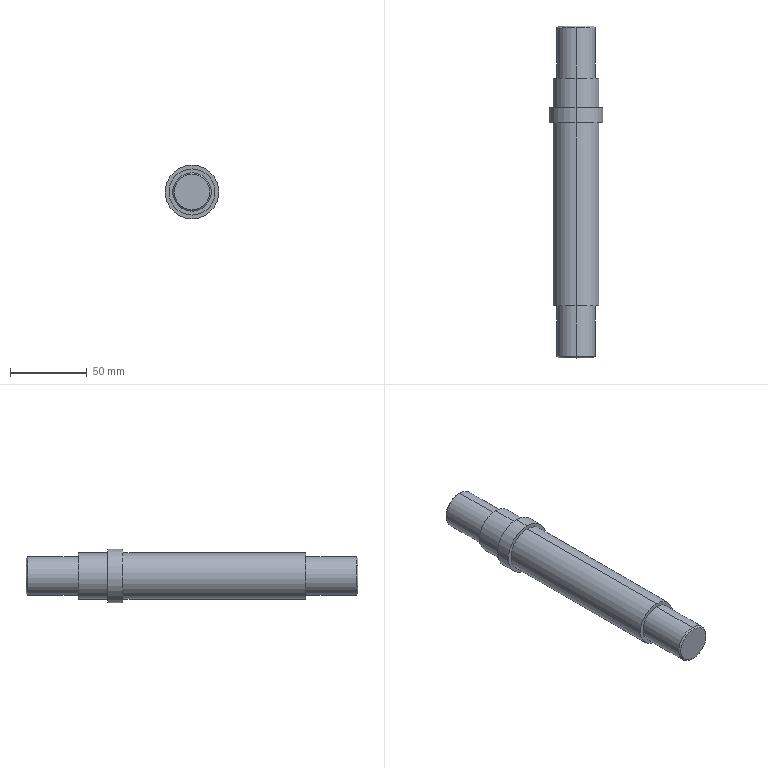Part | STEP file | 012-6-07-04 | 1 solid | 20 faces | box 35 x 216.4 x 35 mm | volume 140753 mm3 | cylinder 10 | plane 6 | cone 4 | commonest cylinder face diameters 25 x4 30 x4 35 x2
STEP:
#1=CARTESIAN_POINT('',(0.,0.,0.));
#2=DIRECTION('',(0.,0.,1.));
#3=DIRECTION('',(1.,0.,0.));
#4=AXIS2_PLACEMENT_3D('',#1,#2,#3);
#5=CARTESIAN_POINT('',(0.,216.4,11.5));
#6=VERTEX_POINT('',#5);
#7=CARTESIAN_POINT('',(0.,216.4,-11.5));
#8=VERTEX_POINT('',#7);
#9=CARTESIAN_POINT('',(0.,216.4,0.));
#10=DIRECTION('',(0.,1.,0.));
#11=DIRECTION('',(0.,0.,1.));
#12=AXIS2_PLACEMENT_3D('',#9,#10,#11);
#13=CIRCLE('',#12,11.5);
#14=CARTESIAN_POINT('',(0.,215.4,0.));
#15=DIRECTION('',(0.,-1.,0.));
#16=DIRECTION('',(0.,0.,-1.));
#17=AXIS2_PLACEMENT_3D('',#14,#15,#16);
#18=CONICAL_SURFACE('',#17,12.5,0.7854);
#19=CARTESIAN_POINT('',(3.142,-1.));
#20=DIRECTION('',(-1.,0.));
#21=VECTOR('',#20,1.);
#22=LINE('',#19,#21);
#23=(GEOMETRIC_REPRESENTATION_CONTEXT(2)PARAMETRIC_REPRESENTATION_CONTEXT()REPRESENTATION_CONTEXT('',''));
#24=DEFINITIONAL_REPRESENTATION('',(#22),#23);
#25=PCURVE('',#18,#24);
#26=CARTESIAN_POINT('',(12.5,216.4,0.));
#27=DIRECTION('',(0.,1.,0.));
#28=DIRECTION('',(0.,0.,1.));
#29=AXIS2_PLACEMENT_3D('',#26,#27,#28);
#30=PLANE('',#29);
#31=CARTESIAN_POINT('',(0.,-12.5));
#32=DIRECTION('',(1.,0.));
#33=AXIS2_PLACEMENT_2D('',#31,#32);
#34=CIRCLE('',#33,11.5);
#35=(GEOMETRIC_REPRESENTATION_CONTEXT(2)PARAMETRIC_REPRESENTATION_CONTEXT()REPRESENTATION_CONTEXT('',''));
#36=DEFINITIONAL_REPRESENTATION('',(#34),#35);
#37=PCURVE('',#30,#36);
#38=SURFACE_CURVE('',#13,(#25,#37),.PCURVE_S1.);
#39=EDGE_CURVE('',#6,#8,#38,.T.);
#40=ORIENTED_EDGE('',*,*,#39,.F.);
#41=CARTESIAN_POINT('',(0.,215.4,12.5));
#42=VERTEX_POINT('',#41);
#43=CARTESIAN_POINT('',(0.,215.4,12.5));
#44=DIRECTION('',(0.,-0.7071,0.7071));
#45=VECTOR('',#44,1.);
#46=LINE('',#43,#45);
#47=CARTESIAN_POINT('',(3.142,0.));
#48=DIRECTION('',(0.,1.));
#49=VECTOR('',#48,1.);
#50=LINE('',#47,#49);
#51=(GEOMETRIC_REPRESENTATION_CONTEXT(2)PARAMETRIC_REPRESENTATION_CONTEXT()REPRESENTATION_CONTEXT('',''));
#52=DEFINITIONAL_REPRESENTATION('',(#50),#51);
#53=PCURVE('',#18,#52);
#54=CARTESIAN_POINT('',(0.,215.4,0.));
#55=DIRECTION('',(0.,-1.,0.));
#56=DIRECTION('',(0.,0.,-1.));
#57=AXIS2_PLACEMENT_3D('',#54,#55,#56);
#58=CONICAL_SURFACE('',#57,12.5,0.7854);
#59=CARTESIAN_POINT('',(3.142,0.));
#60=DIRECTION('',(0.,1.));
#61=VECTOR('',#60,1.);
#62=LINE('',#59,#61);
#63=(GEOMETRIC_REPRESENTATION_CONTEXT(2)PARAMETRIC_REPRESENTATION_CONTEXT()REPRESENTATION_CONTEXT('',''));
#64=DEFINITIONAL_REPRESENTATION('',(#62),#63);
#65=PCURVE('',#58,#64);
#66=SURFACE_CURVE('',#46,(#53,#65),.PCURVE_S1.);
#67=EDGE_CURVE('',#6,#42,#66,.T.);
#68=ORIENTED_EDGE('',*,*,#67,.T.);
#69=CARTESIAN_POINT('',(0.,215.4,-12.5));
#70=VERTEX_POINT('',#69);
#71=CARTESIAN_POINT('',(0.,215.4,0.));
#72=DIRECTION('',(0.,-1.,0.));
#73=DIRECTION('',(0.,0.,1.));
#74=AXIS2_PLACEMENT_3D('',#71,#72,#73);
#75=CIRCLE('',#74,12.5);
#76=CARTESIAN_POINT('',(-3.142,0.));
#77=DIRECTION('',(1.,0.));
#78=VECTOR('',#77,1.);
#79=LINE('',#76,#78);
#80=(GEOMETRIC_REPRESENTATION_CONTEXT(2)PARAMETRIC_REPRESENTATION_CONTEXT()REPRESENTATION_CONTEXT('',''));
#81=DEFINITIONAL_REPRESENTATION('',(#79),#80);
#82=PCURVE('',#18,#81);
#83=CARTESIAN_POINT('',(0.,0.,0.));
#84=DIRECTION('',(0.,-1.,0.));
#85=DIRECTION('',(0.,0.,-1.));
#86=AXIS2_PLACEMENT_3D('',#83,#84,#85);
#87=CYLINDRICAL_SURFACE('',#86,12.5);
#88=CARTESIAN_POINT('',(-3.142,-215.4));
#89=DIRECTION('',(1.,0.));
#90=VECTOR('',#89,1.);
#91=LINE('',#88,#90);
#92=(GEOMETRIC_REPRESENTATION_CONTEXT(2)PARAMETRIC_REPRESENTATION_CONTEXT()REPRESENTATION_CONTEXT('',''));
#93=DEFINITIONAL_REPRESENTATION('',(#91),#92);
#94=PCURVE('',#87,#93);
#95=SURFACE_CURVE('',#75,(#82,#94),.PCURVE_S1.);
#96=EDGE_CURVE('',#70,#42,#95,.T.);
#97=ORIENTED_EDGE('',*,*,#96,.F.);
#98=CARTESIAN_POINT('',(0.,215.4,-12.5));
#99=DIRECTION('',(0.,-0.7071,-0.7071));
#100=VECTOR('',#99,1.);
#101=LINE('',#98,#100);
#102=CARTESIAN_POINT('',(0.,0.));
#103=DIRECTION('',(0.,1.));
#104=VECTOR('',#103,1.);
#105=LINE('',#102,#104);
#106=(GEOMETRIC_REPRESENTATION_CONTEXT(2)PARAMETRIC_REPRESENTATION_CONTEXT()REPRESENTATION_CONTEXT('',''));
#107=DEFINITIONAL_REPRESENTATION('',(#105),#106);
#108=PCURVE('',#18,#107);
#109=CARTESIAN_POINT('',(6.283,0.));
#110=DIRECTION('',(0.,1.));
#111=VECTOR('',#110,1.);
#112=LINE('',#109,#111);
#113=(GEOMETRIC_REPRESENTATION_CONTEXT(2)PARAMETRIC_REPRESENTATION_CONTEXT()REPRESENTATION_CONTEXT('',''));
#114=DEFINITIONAL_REPRESENTATION('',(#112),#113);
#115=PCURVE('',#58,#114);
#116=SURFACE_CURVE('',#101,(#108,#115),.PCURVE_S1.);
#117=EDGE_CURVE('',#8,#70,#116,.T.);
#118=ORIENTED_EDGE('',*,*,#117,.F.);
#119=EDGE_LOOP('',(#40,#68,#97,#118));
#120=FACE_BOUND('',#119,.T.);
#121=ADVANCED_FACE('',(#120),#18,.T.);
#122=CARTESIAN_POINT('',(0.,0.,-11.5));
#123=VERTEX_POINT('',#122);
#124=CARTESIAN_POINT('',(0.,0.,11.5));
#125=VERTEX_POINT('',#124);
#126=CARTESIAN_POINT('',(0.,0.,0.));
#127=DIRECTION('',(0.,-1.,0.));
#128=DIRECTION('',(0.,0.,-1.));
#129=AXIS2_PLACEMENT_3D('',#126,#127,#128);
#130=CIRCLE('',#129,11.5);
#131=CARTESIAN_POINT('',(0.,0.,0.));
#132=DIRECTION('',(0.,1.,0.));
#133=DIRECTION('',(0.,0.,1.));
#134=AXIS2_PLACEMENT_3D('',#131,#132,#133);
#135=CONICAL_SURFACE('',#134,11.5,0.7854);
#136=CARTESIAN_POINT('',(3.142,0.));
#137=DIRECTION('',(-1.,0.));
#138=VECTOR('',#137,1.);
#139=LINE('',#136,#138);
#140=(GEOMETRIC_REPRESENTATION_CONTEXT(2)PARAMETRIC_REPRESENTATION_CONTEXT()REPRESENTATION_CONTEXT('',''));
#141=DEFINITIONAL_REPRESENTATION('',(#139),#140);
#142=PCURVE('',#135,#141);
#143=CARTESIAN_POINT('',(0.,0.,0.));
#144=DIRECTION('',(0.,-1.,0.));
#145=DIRECTION('',(0.,0.,-1.));
#146=AXIS2_PLACEMENT_3D('',#143,#144,#145);
#147=PLANE('',#146);
#148=CARTESIAN_POINT('',(0.,0.));
#149=DIRECTION('',(1.,0.));
#150=AXIS2_PLACEMENT_2D('',#148,#149);
#151=CIRCLE('',#150,11.5);
#152=(GEOMETRIC_REPRESENTATION_CONTEXT(2)PARAMETRIC_REPRESENTATION_CONTEXT()REPRESENTATION_CONTEXT('',''));
#153=DEFINITIONAL_REPRESENTATION('',(#151),#152);
#154=PCURVE('',#147,#153);
#155=SURFACE_CURVE('',#130,(#142,#154),.PCURVE_S1.);
#156=EDGE_CURVE('',#123,#125,#155,.T.);
#157=ORIENTED_EDGE('',*,*,#156,.F.);
#158=CARTESIAN_POINT('',(0.,1.,-12.5));
#159=VERTEX_POINT('',#158);
#160=CARTESIAN_POINT('',(0.,0.,-11.5));
#161=DIRECTION('',(0.,0.7071,-0.7071));
#162=VECTOR('',#161,1.);
#163=LINE('',#160,#162);
#164=CARTESIAN_POINT('',(3.142,0.));
#165=DIRECTION('',(0.,1.));
#166=VECTOR('',#165,1.);
#167=LINE('',#164,#166);
#168=(GEOMETRIC_REPRESENTATION_CONTEXT(2)PARAMETRIC_REPRESENTATION_CONTEXT()REPRESENTATION_CONTEXT('',''));
#169=DEFINITIONAL_REPRESENTATION('',(#167),#168);
#170=PCURVE('',#135,#169);
#171=CARTESIAN_POINT('',(0.,0.,0.));
#172=DIRECTION('',(0.,1.,0.));
#173=DIRECTION('',(0.,0.,1.));
#174=AXIS2_PLACEMENT_3D('',#171,#172,#173);
#175=CONICAL_SURFACE('',#174,11.5,0.7854);
#176=CARTESIAN_POINT('',(3.142,0.));
#177=DIRECTION('',(0.,1.));
#178=VECTOR('',#177,1.);
#179=LINE('',#176,#178);
#180=(GEOMETRIC_REPRESENTATION_CONTEXT(2)PARAMETRIC_REPRESENTATION_CONTEXT()REPRESENTATION_CONTEXT('',''));
#181=DEFINITIONAL_REPRESENTATION('',(#179),#180);
#182=PCURVE('',#175,#181);
#183=SURFACE_CURVE('',#163,(#170,#182),.PCURVE_S1.);
#184=EDGE_CURVE('',#123,#159,#183,.T.);
#185=ORIENTED_EDGE('',*,*,#184,.T.);
#186=CARTESIAN_POINT('',(0.,1.,12.5));
#187=VERTEX_POINT('',#186);
#188=CARTESIAN_POINT('',(0.,1.,0.));
#189=DIRECTION('',(0.,1.,0.));
#190=DIRECTION('',(0.,0.,-1.));
#191=AXIS2_PLACEMENT_3D('',#188,#189,#190);
#192=CIRCLE('',#191,12.5);
#193=CARTESIAN_POINT('',(-3.142,1.));
#194=DIRECTION('',(1.,0.));
#195=VECTOR('',#194,1.);
#196=LINE('',#193,#195);
#197=(GEOMETRIC_REPRESENTATION_CONTEXT(2)PARAMETRIC_REPRESENTATION_CONTEXT()REPRESENTATION_CONTEXT('',''));
#198=DEFINITIONAL_REPRESENTATION('',(#196),#197);
#199=PCURVE('',#135,#198);
#200=CARTESIAN_POINT('',(0.,0.,0.));
#201=DIRECTION('',(0.,-1.,0.));
#202=DIRECTION('',(0.,0.,-1.));
#203=AXIS2_PLACEMENT_3D('',#200,#201,#202);
#204=CYLINDRICAL_SURFACE('',#203,12.5);
#205=CARTESIAN_POINT('',(6.283,-1.));
#206=DIRECTION('',(-1.,0.));
#207=VECTOR('',#206,1.);
#208=LINE('',#205,#207);
#209=(GEOMETRIC_REPRESENTATION_CONTEXT(2)PARAMETRIC_REPRESENTATION_CONTEXT()REPRESENTATION_CONTEXT('',''));
#210=DEFINITIONAL_REPRESENTATION('',(#208),#209);
#211=PCURVE('',#204,#210);
#212=SURFACE_CURVE('',#192,(#199,#211),.PCURVE_S1.);
#213=EDGE_CURVE('',#187,#159,#212,.T.);
#214=ORIENTED_EDGE('',*,*,#213,.F.);
#215=CARTESIAN_POINT('',(0.,0.,11.5));
#216=DIRECTION('',(0.,0.7071,0.7071));
#217=VECTOR('',#216,1.);
#218=LINE('',#215,#217);
#219=CARTESIAN_POINT('',(0.,0.));
#220=DIRECTION('',(0.,1.));
#221=VECTOR('',#220,1.);
#222=LINE('',#219,#221);
#223=(GEOMETRIC_REPRESENTATION_CONTEXT(2)PARAMETRIC_REPRESENTATION_CONTEXT()REPRESENTATION_CONTEXT('',''));
#224=DEFINITIONAL_REPRESENTATION('',(#222),#223);
#225=PCURVE('',#135,#224);
#226=CARTESIAN_POINT('',(6.283,0.));
#227=DIRECTION('',(0.,1.));
#228=VECTOR('',#227,1.);
#229=LINE('',#226,#228);
#230=(GEOMETRIC_REPRESENTATION_CONTEXT(2)PARAMETRIC_REPRESENTATION_CONTEXT()REPRESENTATION_CONTEXT('',''));
#231=DEFINITIONAL_REPRESENTATION('',(#229),#230);
#232=PCURVE('',#175,#231);
#233=SURFACE_CURVE('',#218,(#225,#232),.PCURVE_S1.);
#234=EDGE_CURVE('',#125,#187,#233,.T.);
#235=ORIENTED_EDGE('',*,*,#234,.F.);
#236=EDGE_LOOP('',(#157,#185,#214,#235));
#237=FACE_BOUND('',#236,.T.);
#238=ADVANCED_FACE('',(#237),#135,.T.);
#239=ORIENTED_EDGE('',*,*,#96,.T.);
#240=CARTESIAN_POINT('',(0.,182.4,12.5));
#241=VERTEX_POINT('',#240);
#242=CARTESIAN_POINT('',(0.,0.,12.5));
#243=DIRECTION('',(0.,-1.,0.));
#244=VECTOR('',#243,1.);
#245=LINE('',#242,#244);
#246=CARTESIAN_POINT('',(3.142,0.));
#247=DIRECTION('',(0.,1.));
#248=VECTOR('',#247,1.);
#249=LINE('',#246,#248);
#250=(GEOMETRIC_REPRESENTATION_CONTEXT(2)PARAMETRIC_REPRESENTATION_CONTEXT()REPRESENTATION_CONTEXT('',''));
#251=DEFINITIONAL_REPRESENTATION('',(#249),#250);
#252=PCURVE('',#87,#251);
#253=CARTESIAN_POINT('',(0.,0.,0.));
#254=DIRECTION('',(0.,-1.,0.));
#255=DIRECTION('',(0.,0.,-1.));
#256=AXIS2_PLACEMENT_3D('',#253,#254,#255);
#257=CYLINDRICAL_SURFACE('',#256,12.5);
#258=CARTESIAN_POINT('',(3.142,0.));
#259=DIRECTION('',(0.,1.));
#260=VECTOR('',#259,1.);
#261=LINE('',#258,#260);
#262=(GEOMETRIC_REPRESENTATION_CONTEXT(2)PARAMETRIC_REPRESENTATION_CONTEXT()REPRESENTATION_CONTEXT('',''));
#263=DEFINITIONAL_REPRESENTATION('',(#261),#262);
#264=PCURVE('',#257,#263);
#265=SURFACE_CURVE('',#245,(#252,#264),.PCURVE_S1.);
#266=EDGE_CURVE('',#42,#241,#265,.T.);
#267=ORIENTED_EDGE('',*,*,#266,.T.);
#268=CARTESIAN_POINT('',(0.,182.4,-12.5));
#269=VERTEX_POINT('',#268);
#270=CARTESIAN_POINT('',(0.,182.4,0.));
#271=DIRECTION('',(0.,-1.,0.));
#272=DIRECTION('',(0.,0.,-1.));
#273=AXIS2_PLACEMENT_3D('',#270,#271,#272);
#274=CIRCLE('',#273,12.5);
#275=CARTESIAN_POINT('',(0.,-182.4));
#276=DIRECTION('',(1.,0.));
#277=VECTOR('',#276,1.);
#278=LINE('',#275,#277);
#279=(GEOMETRIC_REPRESENTATION_CONTEXT(2)PARAMETRIC_REPRESENTATION_CONTEXT()REPRESENTATION_CONTEXT('',''));
#280=DEFINITIONAL_REPRESENTATION('',(#278),#279);
#281=PCURVE('',#87,#280);
#282=CARTESIAN_POINT('',(12.5,182.4,0.));
#283=DIRECTION('',(0.,1.,0.));
#284=DIRECTION('',(0.,0.,1.));
#285=AXIS2_PLACEMENT_3D('',#282,#283,#284);
#286=PLANE('',#285);
#287=CARTESIAN_POINT('',(-12.5,-12.5));
#288=CARTESIAN_POINT('',(-12.5,9.151));
#289=CARTESIAN_POINT('',(6.25,-1.675));
#290=CARTESIAN_POINT('',(25.,-12.5));
#291=CARTESIAN_POINT('',(6.25,-23.325));
#292=CARTESIAN_POINT('',(-12.5,-34.151));
#293=CARTESIAN_POINT('',(-12.5,-12.5));
#294=(BOUNDED_CURVE()B_SPLINE_CURVE(2,(#287,#288,#289,#290,#291,#292,#293),.UNSPECIFIED.,.T.,.F.)B_SPLINE_CURVE_WITH_KNOTS((1,2,2,2,2,1),(-2.094,0.,2.094,4.189,6.283,8.378),.UNSPECIFIED.)CURVE()GEOMETRIC_REPRESENTATION_ITEM()RATIONAL_B_SPLINE_CURVE((1.,0.5,1.,0.5,1.,0.5,1.))REPRESENTATION_ITEM(''));
#295=(GEOMETRIC_REPRESENTATION_CONTEXT(2)PARAMETRIC_REPRESENTATION_CONTEXT()REPRESENTATION_CONTEXT('',''));
#296=DEFINITIONAL_REPRESENTATION('',(#294),#295);
#297=PCURVE('',#286,#296);
#298=SURFACE_CURVE('',#274,(#281,#297),.PCURVE_S1.);
#299=EDGE_CURVE('',#269,#241,#298,.T.);
#300=ORIENTED_EDGE('',*,*,#299,.F.);
#301=CARTESIAN_POINT('',(0.,0.,-12.5));
#302=DIRECTION('',(0.,-1.,0.));
#303=VECTOR('',#302,1.);
#304=LINE('',#301,#303);
#305=CARTESIAN_POINT('',(0.,0.));
#306=DIRECTION('',(0.,1.));
#307=VECTOR('',#306,1.);
#308=LINE('',#305,#307);
#309=(GEOMETRIC_REPRESENTATION_CONTEXT(2)PARAMETRIC_REPRESENTATION_CONTEXT()REPRESENTATION_CONTEXT('',''));
#310=DEFINITIONAL_REPRESENTATION('',(#308),#309);
#311=PCURVE('',#87,#310);
#312=CARTESIAN_POINT('',(6.283,0.));
#313=DIRECTION('',(0.,1.));
#314=VECTOR('',#313,1.);
#315=LINE('',#312,#314);
#316=(GEOMETRIC_REPRESENTATION_CONTEXT(2)PARAMETRIC_REPRESENTATION_CONTEXT()REPRESENTATION_CONTEXT('',''));
#317=DEFINITIONAL_REPRESENTATION('',(#315),#316);
#318=PCURVE('',#257,#317);
#319=SURFACE_CURVE('',#304,(#311,#318),.PCURVE_S1.);
#320=EDGE_CURVE('',#70,#269,#319,.T.);
#321=ORIENTED_EDGE('',*,*,#320,.F.);
#322=EDGE_LOOP('',(#239,#267,#300,#321));
#323=FACE_BOUND('',#322,.T.);
#324=ADVANCED_FACE('',(#323),#87,.T.);
#325=CARTESIAN_POINT('',(0.,182.4,-15.));
#326=VERTEX_POINT('',#325);
#327=CARTESIAN_POINT('',(0.,182.4,15.));
#328=VERTEX_POINT('',#327);
#329=CARTESIAN_POINT('',(0.,182.4,0.));
#330=DIRECTION('',(0.,-1.,0.));
#331=DIRECTION('',(0.,0.,-1.));
#332=AXIS2_PLACEMENT_3D('',#329,#330,#331);
#333=CIRCLE('',#332,15.);
#334=CARTESIAN_POINT('',(0.,0.,0.));
#335=DIRECTION('',(0.,-1.,0.));
#336=DIRECTION('',(0.,0.,-1.));
#337=AXIS2_PLACEMENT_3D('',#334,#335,#336);
#338=CYLINDRICAL_SURFACE('',#337,15.);
#339=CARTESIAN_POINT('',(0.,-182.4));
#340=DIRECTION('',(1.,0.));
#341=VECTOR('',#340,1.);
#342=LINE('',#339,#341);
#343=(GEOMETRIC_REPRESENTATION_CONTEXT(2)PARAMETRIC_REPRESENTATION_CONTEXT()REPRESENTATION_CONTEXT('',''));
#344=DEFINITIONAL_REPRESENTATION('',(#342),#343);
#345=PCURVE('',#338,#344);
#346=CARTESIAN_POINT('',(-15.,-12.5));
#347=CARTESIAN_POINT('',(-15.,13.481));
#348=CARTESIAN_POINT('',(7.5,0.4904));
#349=CARTESIAN_POINT('',(30.,-12.5));
#350=CARTESIAN_POINT('',(7.5,-25.49));
#351=CARTESIAN_POINT('',(-15.,-38.481));
#352=CARTESIAN_POINT('',(-15.,-12.5));
#353=(BOUNDED_CURVE()B_SPLINE_CURVE(2,(#346,#347,#348,#349,#350,#351,#352),.UNSPECIFIED.,.T.,.F.)B_SPLINE_CURVE_WITH_KNOTS((1,2,2,2,2,1),(-2.094,0.,2.094,4.189,6.283,8.378),.UNSPECIFIED.)CURVE()GEOMETRIC_REPRESENTATION_ITEM()RATIONAL_B_SPLINE_CURVE((1.,0.5,1.,0.5,1.,0.5,1.))REPRESENTATION_ITEM(''));
#354=(GEOMETRIC_REPRESENTATION_CONTEXT(2)PARAMETRIC_REPRESENTATION_CONTEXT()REPRESENTATION_CONTEXT('',''));
#355=DEFINITIONAL_REPRESENTATION('',(#353),#354);
#356=PCURVE('',#286,#355);
#357=SURFACE_CURVE('',#333,(#345,#356),.PCURVE_S1.);
#358=EDGE_CURVE('',#326,#328,#357,.T.);
#359=ORIENTED_EDGE('',*,*,#358,.T.);
#360=CARTESIAN_POINT('',(0.,163.2,15.));
#361=VERTEX_POINT('',#360);
#362=CARTESIAN_POINT('',(0.,0.,15.));
#363=DIRECTION('',(0.,-1.,0.));
#364=VECTOR('',#363,1.);
#365=LINE('',#362,#364);
#366=CARTESIAN_POINT('',(3.142,0.));
#367=DIRECTION('',(0.,1.));
#368=VECTOR('',#367,1.);
#369=LINE('',#366,#368);
#370=(GEOMETRIC_REPRESENTATION_CONTEXT(2)PARAMETRIC_REPRESENTATION_CONTEXT()REPRESENTATION_CONTEXT('',''));
#371=DEFINITIONAL_REPRESENTATION('',(#369),#370);
#372=PCURVE('',#338,#371);
#373=CARTESIAN_POINT('',(0.,0.,0.));
#374=DIRECTION('',(0.,-1.,0.));
#375=DIRECTION('',(0.,0.,-1.));
#376=AXIS2_PLACEMENT_3D('',#373,#374,#375);
#377=CYLINDRICAL_SURFACE('',#376,15.);
#378=CARTESIAN_POINT('',(3.142,0.));
#379=DIRECTION('',(0.,1.));
#380=VECTOR('',#379,1.);
#381=LINE('',#378,#380);
#382=(GEOMETRIC_REPRESENTATION_CONTEXT(2)PARAMETRIC_REPRESENTATION_CONTEXT()REPRESENTATION_CONTEXT('',''));
#383=DEFINITIONAL_REPRESENTATION('',(#381),#382);
#384=PCURVE('',#377,#383);
#385=SURFACE_CURVE('',#365,(#372,#384),.PCURVE_S1.);
#386=EDGE_CURVE('',#328,#361,#385,.T.);
#387=ORIENTED_EDGE('',*,*,#386,.T.);
#388=CARTESIAN_POINT('',(0.,163.2,-15.));
#389=VERTEX_POINT('',#388);
#390=CARTESIAN_POINT('',(0.,163.2,0.));
#391=DIRECTION('',(0.,-1.,0.));
#392=DIRECTION('',(0.,0.,-1.));
#393=AXIS2_PLACEMENT_3D('',#390,#391,#392);
#394=CIRCLE('',#393,15.);
#395=CARTESIAN_POINT('',(0.,-163.2));
#396=DIRECTION('',(1.,0.));
#397=VECTOR('',#396,1.);
#398=LINE('',#395,#397);
#399=(GEOMETRIC_REPRESENTATION_CONTEXT(2)PARAMETRIC_REPRESENTATION_CONTEXT()REPRESENTATION_CONTEXT('',''));
#400=DEFINITIONAL_REPRESENTATION('',(#398),#399);
#401=PCURVE('',#338,#400);
#402=CARTESIAN_POINT('',(15.,163.2,0.));
#403=DIRECTION('',(0.,1.,0.));
#404=DIRECTION('',(0.,0.,1.));
#405=AXIS2_PLACEMENT_3D('',#402,#403,#404);
#406=PLANE('',#405);
#407=CARTESIAN_POINT('',(-15.,-15.));
#408=CARTESIAN_POINT('',(-15.,10.981));
#409=CARTESIAN_POINT('',(7.5,-2.01));
#410=CARTESIAN_POINT('',(30.,-15.));
#411=CARTESIAN_POINT('',(7.5,-27.99));
#412=CARTESIAN_POINT('',(-15.,-40.981));
#413=CARTESIAN_POINT('',(-15.,-15.));
#414=(BOUNDED_CURVE()B_SPLINE_CURVE(2,(#407,#408,#409,#410,#411,#412,#413),.UNSPECIFIED.,.T.,.F.)B_SPLINE_CURVE_WITH_KNOTS((1,2,2,2,2,1),(-2.094,0.,2.094,4.189,6.283,8.378),.UNSPECIFIED.)CURVE()GEOMETRIC_REPRESENTATION_ITEM()RATIONAL_B_SPLINE_CURVE((1.,0.5,1.,0.5,1.,0.5,1.))REPRESENTATION_ITEM(''));
#415=(GEOMETRIC_REPRESENTATION_CONTEXT(2)PARAMETRIC_REPRESENTATION_CONTEXT()REPRESENTATION_CONTEXT('',''));
#416=DEFINITIONAL_REPRESENTATION('',(#414),#415);
#417=PCURVE('',#406,#416);
#418=SURFACE_CURVE('',#394,(#401,#417),.PCURVE_S1.);
#419=EDGE_CURVE('',#389,#361,#418,.T.);
#420=ORIENTED_EDGE('',*,*,#419,.F.);
#421=CARTESIAN_POINT('',(0.,0.,-15.));
#422=DIRECTION('',(0.,-1.,0.));
#423=VECTOR('',#422,1.);
#424=LINE('',#421,#423);
#425=CARTESIAN_POINT('',(0.,0.));
#426=DIRECTION('',(0.,1.));
#427=VECTOR('',#426,1.);
#428=LINE('',#425,#427);
#429=(GEOMETRIC_REPRESENTATION_CONTEXT(2)PARAMETRIC_REPRESENTATION_CONTEXT()REPRESENTATION_CONTEXT('',''));
#430=DEFINITIONAL_REPRESENTATION('',(#428),#429);
#431=PCURVE('',#338,#430);
#432=CARTESIAN_POINT('',(6.283,0.));
#433=DIRECTION('',(0.,1.));
#434=VECTOR('',#433,1.);
#435=LINE('',#432,#434);
#436=(GEOMETRIC_REPRESENTATION_CONTEXT(2)PARAMETRIC_REPRESENTATION_CONTEXT()REPRESENTATION_CONTEXT('',''));
#437=DEFINITIONAL_REPRESENTATION('',(#435),#436);
#438=PCURVE('',#377,#437);
#439=SURFACE_CURVE('',#424,(#431,#438),.PCURVE_S1.);
#440=EDGE_CURVE('',#326,#389,#439,.T.);
#441=ORIENTED_EDGE('',*,*,#440,.F.);
#442=EDGE_LOOP('',(#359,#387,#420,#441));
#443=FACE_BOUND('',#442,.T.);
#444=ADVANCED_FACE('',(#443),#338,.T.);
#445=CARTESIAN_POINT('',(0.,163.2,-17.5));
#446=VERTEX_POINT('',#445);
#447=CARTESIAN_POINT('',(0.,163.2,17.5));
#448=VERTEX_POINT('',#447);
#449=CARTESIAN_POINT('',(0.,163.2,0.));
#450=DIRECTION('',(0.,-1.,0.));
#451=DIRECTION('',(0.,0.,-1.));
#452=AXIS2_PLACEMENT_3D('',#449,#450,#451);
#453=CIRCLE('',#452,17.5);
#454=CARTESIAN_POINT('',(0.,0.,0.));
#455=DIRECTION('',(0.,-1.,0.));
#456=DIRECTION('',(0.,0.,-1.));
#457=AXIS2_PLACEMENT_3D('',#454,#455,#456);
#458=CYLINDRICAL_SURFACE('',#457,17.5);
#459=CARTESIAN_POINT('',(0.,-163.2));
#460=DIRECTION('',(1.,0.));
#461=VECTOR('',#460,1.);
#462=LINE('',#459,#461);
#463=(GEOMETRIC_REPRESENTATION_CONTEXT(2)PARAMETRIC_REPRESENTATION_CONTEXT()REPRESENTATION_CONTEXT('',''));
#464=DEFINITIONAL_REPRESENTATION('',(#462),#463);
#465=PCURVE('',#458,#464);
#466=CARTESIAN_POINT('',(-17.5,-15.));
#467=CARTESIAN_POINT('',(-17.5,15.311));
#468=CARTESIAN_POINT('',(8.75,0.1554));
#469=CARTESIAN_POINT('',(35.,-15.));
#470=CARTESIAN_POINT('',(8.75,-30.155));
#471=CARTESIAN_POINT('',(-17.5,-45.311));
#472=CARTESIAN_POINT('',(-17.5,-15.));
#473=(BOUNDED_CURVE()B_SPLINE_CURVE(2,(#466,#467,#468,#469,#470,#471,#472),.UNSPECIFIED.,.T.,.F.)B_SPLINE_CURVE_WITH_KNOTS((1,2,2,2,2,1),(-2.094,0.,2.094,4.189,6.283,8.378),.UNSPECIFIED.)CURVE()GEOMETRIC_REPRESENTATION_ITEM()RATIONAL_B_SPLINE_CURVE((1.,0.5,1.,0.5,1.,0.5,1.))REPRESENTATION_ITEM(''));
#474=(GEOMETRIC_REPRESENTATION_CONTEXT(2)PARAMETRIC_REPRESENTATION_CONTEXT()REPRESENTATION_CONTEXT('',''));
#475=DEFINITIONAL_REPRESENTATION('',(#473),#474);
#476=PCURVE('',#406,#475);
#477=SURFACE_CURVE('',#453,(#465,#476),.PCURVE_S1.);
#478=EDGE_CURVE('',#446,#448,#477,.T.);
#479=ORIENTED_EDGE('',*,*,#478,.T.);
#480=CARTESIAN_POINT('',(0.,153.2,17.5));
#481=VERTEX_POINT('',#480);
#482=CARTESIAN_POINT('',(0.,0.,17.5));
#483=DIRECTION('',(0.,-1.,0.));
#484=VECTOR('',#483,1.);
#485=LINE('',#482,#484);
#486=CARTESIAN_POINT('',(3.142,0.));
#487=DIRECTION('',(0.,1.));
#488=VECTOR('',#487,1.);
#489=LINE('',#486,#488);
#490=(GEOMETRIC_REPRESENTATION_CONTEXT(2)PARAMETRIC_REPRESENTATION_CONTEXT()REPRESENTATION_CONTEXT('',''));
#491=DEFINITIONAL_REPRESENTATION('',(#489),#490);
#492=PCURVE('',#458,#491);
#493=CARTESIAN_POINT('',(0.,0.,0.));
#494=DIRECTION('',(0.,-1.,0.));
#495=DIRECTION('',(0.,0.,-1.));
#496=AXIS2_PLACEMENT_3D('',#493,#494,#495);
#497=CYLINDRICAL_SURFACE('',#496,17.5);
#498=CARTESIAN_POINT('',(3.142,0.));
#499=DIRECTION('',(0.,1.));
#500=VECTOR('',#499,1.);
#501=LINE('',#498,#500);
#502=(GEOMETRIC_REPRESENTATION_CONTEXT(2)PARAMETRIC_REPRESENTATION_CONTEXT()REPRESENTATION_CONTEXT('',''));
#503=DEFINITIONAL_REPRESENTATION('',(#501),#502);
#504=PCURVE('',#497,#503);
#505=SURFACE_CURVE('',#485,(#492,#504),.PCURVE_S1.);
#506=EDGE_CURVE('',#448,#481,#505,.T.);
#507=ORIENTED_EDGE('',*,*,#506,.T.);
#508=CARTESIAN_POINT('',(0.,153.2,-17.5));
#509=VERTEX_POINT('',#508);
#510=CARTESIAN_POINT('',(0.,153.2,0.));
#511=DIRECTION('',(0.,-1.,0.));
#512=DIRECTION('',(0.,0.,-1.));
#513=AXIS2_PLACEMENT_3D('',#510,#511,#512);
#514=CIRCLE('',#513,17.5);
#515=CARTESIAN_POINT('',(0.,-153.2));
#516=DIRECTION('',(1.,0.));
#517=VECTOR('',#516,1.);
#518=LINE('',#515,#517);
#519=(GEOMETRIC_REPRESENTATION_CONTEXT(2)PARAMETRIC_REPRESENTATION_CONTEXT()REPRESENTATION_CONTEXT('',''));
#520=DEFINITIONAL_REPRESENTATION('',(#518),#519);
#521=PCURVE('',#458,#520);
#522=CARTESIAN_POINT('',(15.,153.2,0.));
#523=DIRECTION('',(0.,-1.,0.));
#524=DIRECTION('',(0.,0.,-1.));
#525=AXIS2_PLACEMENT_3D('',#522,#523,#524);
#526=PLANE('',#525);
#527=CARTESIAN_POINT('',(0.,-15.));
#528=DIRECTION('',(1.,0.));
#529=AXIS2_PLACEMENT_2D('',#527,#528);
#530=CIRCLE('',#529,17.5);
#531=(GEOMETRIC_REPRESENTATION_CONTEXT(2)PARAMETRIC_REPRESENTATION_CONTEXT()REPRESENTATION_CONTEXT('',''));
#532=DEFINITIONAL_REPRESENTATION('',(#530),#531);
#533=PCURVE('',#526,#532);
#534=SURFACE_CURVE('',#514,(#521,#533),.PCURVE_S1.);
#535=EDGE_CURVE('',#509,#481,#534,.T.);
#536=ORIENTED_EDGE('',*,*,#535,.F.);
#537=CARTESIAN_POINT('',(0.,0.,-17.5));
#538=DIRECTION('',(0.,-1.,0.));
#539=VECTOR('',#538,1.);
#540=LINE('',#537,#539);
#541=CARTESIAN_POINT('',(0.,0.));
#542=DIRECTION('',(0.,1.));
#543=VECTOR('',#542,1.);
#544=LINE('',#541,#543);
#545=(GEOMETRIC_REPRESENTATION_CONTEXT(2)PARAMETRIC_REPRESENTATION_CONTEXT()REPRESENTATION_CONTEXT('',''));
#546=DEFINITIONAL_REPRESENTATION('',(#544),#545);
#547=PCURVE('',#458,#546);
#548=CARTESIAN_POINT('',(6.283,0.));
#549=DIRECTION('',(0.,1.));
#550=VECTOR('',#549,1.);
#551=LINE('',#548,#550);
#552=(GEOMETRIC_REPRESENTATION_CONTEXT(2)PARAMETRIC_REPRESENTATION_CONTEXT()REPRESENTATION_CONTEXT('',''));
#553=DEFINITIONAL_REPRESENTATION('',(#551),#552);
#554=PCURVE('',#497,#553);
#555=SURFACE_CURVE('',#540,(#547,#554),.PCURVE_S1.);
#556=EDGE_CURVE('',#446,#509,#555,.T.);
#557=ORIENTED_EDGE('',*,*,#556,.F.);
#558=EDGE_LOOP('',(#479,#507,#536,#557));
#559=FACE_BOUND('',#558,.T.);
#560=ADVANCED_FACE('',(#559),#458,.T.);
#561=CARTESIAN_POINT('',(0.,153.2,-15.));
#562=VERTEX_POINT('',#561);
#563=CARTESIAN_POINT('',(0.,153.2,15.));
#564=VERTEX_POINT('',#563);
#565=CARTESIAN_POINT('',(0.,153.2,0.));
#566=DIRECTION('',(0.,-1.,0.));
#567=DIRECTION('',(0.,0.,-1.));
#568=AXIS2_PLACEMENT_3D('',#565,#566,#567);
#569=CIRCLE('',#568,15.);
#570=CARTESIAN_POINT('',(0.,0.,0.));
#571=DIRECTION('',(0.,-1.,0.));
#572=DIRECTION('',(0.,0.,-1.));
#573=AXIS2_PLACEMENT_3D('',#570,#571,#572);
#574=CYLINDRICAL_SURFACE('',#573,15.);
#575=CARTESIAN_POINT('',(0.,-153.2));
#576=DIRECTION('',(1.,0.));
#577=VECTOR('',#576,1.);
#578=LINE('',#575,#577);
#579=(GEOMETRIC_REPRESENTATION_CONTEXT(2)PARAMETRIC_REPRESENTATION_CONTEXT()REPRESENTATION_CONTEXT('',''));
#580=DEFINITIONAL_REPRESENTATION('',(#578),#579);
#581=PCURVE('',#574,#580);
#582=CARTESIAN_POINT('',(0.,-15.));
#583=DIRECTION('',(1.,0.));
#584=AXIS2_PLACEMENT_2D('',#582,#583);
#585=CIRCLE('',#584,15.);
#586=(GEOMETRIC_REPRESENTATION_CONTEXT(2)PARAMETRIC_REPRESENTATION_CONTEXT()REPRESENTATION_CONTEXT('',''));
#587=DEFINITIONAL_REPRESENTATION('',(#585),#586);
#588=PCURVE('',#526,#587);
#589=SURFACE_CURVE('',#569,(#581,#588),.PCURVE_S1.);
#590=EDGE_CURVE('',#562,#564,#589,.T.);
#591=ORIENTED_EDGE('',*,*,#590,.T.);
#592=CARTESIAN_POINT('',(0.,34.,15.));
#593=VERTEX_POINT('',#592);
#594=CARTESIAN_POINT('',(0.,0.,15.));
#595=DIRECTION('',(0.,-1.,0.));
#596=VECTOR('',#595,1.);
#597=LINE('',#594,#596);
#598=CARTESIAN_POINT('',(3.142,0.));
#599=DIRECTION('',(0.,1.));
#600=VECTOR('',#599,1.);
#601=LINE('',#598,#600);
#602=(GEOMETRIC_REPRESENTATION_CONTEXT(2)PARAMETRIC_REPRESENTATION_CONTEXT()REPRESENTATION_CONTEXT('',''));
#603=DEFINITIONAL_REPRESENTATION('',(#601),#602);
#604=PCURVE('',#574,#603);
#605=CARTESIAN_POINT('',(0.,0.,0.));
#606=DIRECTION('',(0.,-1.,0.));
#607=DIRECTION('',(0.,0.,-1.));
#608=AXIS2_PLACEMENT_3D('',#605,#606,#607);
#609=CYLINDRICAL_SURFACE('',#608,15.);
#610=CARTESIAN_POINT('',(3.142,0.));
#611=DIRECTION('',(0.,1.));
#612=VECTOR('',#611,1.);
#613=LINE('',#610,#612);
#614=(GEOMETRIC_REPRESENTATION_CONTEXT(2)PARAMETRIC_REPRESENTATION_CONTEXT()REPRESENTATION_CONTEXT('',''));
#615=DEFINITIONAL_REPRESENTATION('',(#613),#614);
#616=PCURVE('',#609,#615);
#617=SURFACE_CURVE('',#597,(#604,#616),.PCURVE_S1.);
#618=EDGE_CURVE('',#564,#593,#617,.T.);
#619=ORIENTED_EDGE('',*,*,#618,.T.);
#620=CARTESIAN_POINT('',(0.,34.,-15.));
#621=VERTEX_POINT('',#620);
#622=CARTESIAN_POINT('',(0.,34.,0.));
#623=DIRECTION('',(0.,-1.,0.));
#624=DIRECTION('',(0.,0.,-1.));
#625=AXIS2_PLACEMENT_3D('',#622,#623,#624);
#626=CIRCLE('',#625,15.);
#627=CARTESIAN_POINT('',(0.,-34.));
#628=DIRECTION('',(1.,0.));
#629=VECTOR('',#628,1.);
#630=LINE('',#627,#629);
#631=(GEOMETRIC_REPRESENTATION_CONTEXT(2)PARAMETRIC_REPRESENTATION_CONTEXT()REPRESENTATION_CONTEXT('',''));
#632=DEFINITIONAL_REPRESENTATION('',(#630),#631);
#633=PCURVE('',#574,#632);
#634=CARTESIAN_POINT('',(12.5,34.,0.));
#635=DIRECTION('',(0.,-1.,0.));
#636=DIRECTION('',(0.,0.,-1.));
#637=AXIS2_PLACEMENT_3D('',#634,#635,#636);
#638=PLANE('',#637);
#639=CARTESIAN_POINT('',(0.,-12.5));
#640=DIRECTION('',(1.,0.));
#641=AXIS2_PLACEMENT_2D('',#639,#640);
#642=CIRCLE('',#641,15.);
#643=(GEOMETRIC_REPRESENTATION_CONTEXT(2)PARAMETRIC_REPRESENTATION_CONTEXT()REPRESENTATION_CONTEXT('',''));
#644=DEFINITIONAL_REPRESENTATION('',(#642),#643);
#645=PCURVE('',#638,#644);
#646=SURFACE_CURVE('',#626,(#633,#645),.PCURVE_S1.);
#647=EDGE_CURVE('',#621,#593,#646,.T.);
#648=ORIENTED_EDGE('',*,*,#647,.F.);
#649=CARTESIAN_POINT('',(0.,0.,-15.));
#650=DIRECTION('',(0.,-1.,0.));
#651=VECTOR('',#650,1.);
#652=LINE('',#649,#651);
#653=CARTESIAN_POINT('',(0.,0.));
#654=DIRECTION('',(0.,1.));
#655=VECTOR('',#654,1.);
#656=LINE('',#653,#655);
#657=(GEOMETRIC_REPRESENTATION_CONTEXT(2)PARAMETRIC_REPRESENTATION_CONTEXT()REPRESENTATION_CONTEXT('',''));
#658=DEFINITIONAL_REPRESENTATION('',(#656),#657);
#659=PCURVE('',#574,#658);
#660=CARTESIAN_POINT('',(6.283,0.));
#661=DIRECTION('',(0.,1.));
#662=VECTOR('',#661,1.);
#663=LINE('',#660,#662);
#664=(GEOMETRIC_REPRESENTATION_CONTEXT(2)PARAMETRIC_REPRESENTATION_CONTEXT()REPRESENTATION_CONTEXT('',''));
#665=DEFINITIONAL_REPRESENTATION('',(#663),#664);
#666=PCURVE('',#609,#665);
#667=SURFACE_CURVE('',#652,(#659,#666),.PCURVE_S1.);
#668=EDGE_CURVE('',#562,#621,#667,.T.);
#669=ORIENTED_EDGE('',*,*,#668,.F.);
#670=EDGE_LOOP('',(#591,#619,#648,#669));
#671=FACE_BOUND('',#670,.T.);
#672=ADVANCED_FACE('',(#671),#574,.T.);
#673=CARTESIAN_POINT('',(0.,34.,-12.5));
#674=VERTEX_POINT('',#673);
#675=CARTESIAN_POINT('',(0.,34.,12.5));
#676=VERTEX_POINT('',#675);
#677=CARTESIAN_POINT('',(0.,34.,0.));
#678=DIRECTION('',(0.,-1.,0.));
#679=DIRECTION('',(0.,0.,-1.));
#680=AXIS2_PLACEMENT_3D('',#677,#678,#679);
#681=CIRCLE('',#680,12.5);
#682=CARTESIAN_POINT('',(0.,-34.));
#683=DIRECTION('',(1.,0.));
#684=VECTOR('',#683,1.);
#685=LINE('',#682,#684);
#686=(GEOMETRIC_REPRESENTATION_CONTEXT(2)PARAMETRIC_REPRESENTATION_CONTEXT()REPRESENTATION_CONTEXT('',''));
#687=DEFINITIONAL_REPRESENTATION('',(#685),#686);
#688=PCURVE('',#204,#687);
#689=CARTESIAN_POINT('',(0.,-12.5));
#690=DIRECTION('',(1.,0.));
#691=AXIS2_PLACEMENT_2D('',#689,#690);
#692=CIRCLE('',#691,12.5);
#693=(GEOMETRIC_REPRESENTATION_CONTEXT(2)PARAMETRIC_REPRESENTATION_CONTEXT()REPRESENTATION_CONTEXT('',''));
#694=DEFINITIONAL_REPRESENTATION('',(#692),#693);
#695=PCURVE('',#638,#694);
#696=SURFACE_CURVE('',#681,(#688,#695),.PCURVE_S1.);
#697=EDGE_CURVE('',#674,#676,#696,.T.);
#698=ORIENTED_EDGE('',*,*,#697,.T.);
#699=CARTESIAN_POINT('',(0.,0.,12.5));
#700=DIRECTION('',(0.,-1.,0.));
#701=VECTOR('',#700,1.);
#702=LINE('',#699,#701);
#703=CARTESIAN_POINT('',(3.142,0.));
#704=DIRECTION('',(0.,1.));
#705=VECTOR('',#704,1.);
#706=LINE('',#703,#705);
#707=(GEOMETRIC_REPRESENTATION_CONTEXT(2)PARAMETRIC_REPRESENTATION_CONTEXT()REPRESENTATION_CONTEXT('',''));
#708=DEFINITIONAL_REPRESENTATION('',(#706),#707);
#709=PCURVE('',#204,#708);
#710=CARTESIAN_POINT('',(0.,0.,0.));
#711=DIRECTION('',(0.,-1.,0.));
#712=DIRECTION('',(0.,0.,-1.));
#713=AXIS2_PLACEMENT_3D('',#710,#711,#712);
#714=CYLINDRICAL_SURFACE('',#713,12.5);
#715=CARTESIAN_POINT('',(3.142,0.));
#716=DIRECTION('',(0.,1.));
#717=VECTOR('',#716,1.);
#718=LINE('',#715,#717);
#719=(GEOMETRIC_REPRESENTATION_CONTEXT(2)PARAMETRIC_REPRESENTATION_CONTEXT()REPRESENTATION_CONTEXT('',''));
#720=DEFINITIONAL_REPRESENTATION('',(#718),#719);
#721=PCURVE('',#714,#720);
#722=SURFACE_CURVE('',#702,(#709,#721),.PCURVE_S1.);
#723=EDGE_CURVE('',#676,#187,#722,.T.);
#724=ORIENTED_EDGE('',*,*,#723,.T.);
#725=ORIENTED_EDGE('',*,*,#213,.T.);
#726=CARTESIAN_POINT('',(0.,0.,-12.5));
#727=DIRECTION('',(0.,-1.,0.));
#728=VECTOR('',#727,1.);
#729=LINE('',#726,#728);
#730=CARTESIAN_POINT('',(0.,0.));
#731=DIRECTION('',(0.,1.));
#732=VECTOR('',#731,1.);
#733=LINE('',#730,#732);
#734=(GEOMETRIC_REPRESENTATION_CONTEXT(2)PARAMETRIC_REPRESENTATION_CONTEXT()REPRESENTATION_CONTEXT('',''));
#735=DEFINITIONAL_REPRESENTATION('',(#733),#734);
#736=PCURVE('',#204,#735);
#737=CARTESIAN_POINT('',(6.283,0.));
#738=DIRECTION('',(0.,1.));
#739=VECTOR('',#738,1.);
#740=LINE('',#737,#739);
#741=(GEOMETRIC_REPRESENTATION_CONTEXT(2)PARAMETRIC_REPRESENTATION_CONTEXT()REPRESENTATION_CONTEXT('',''));
#742=DEFINITIONAL_REPRESENTATION('',(#740),#741);
#743=PCURVE('',#714,#742);
#744=SURFACE_CURVE('',#729,(#736,#743),.PCURVE_S1.);
#745=EDGE_CURVE('',#674,#159,#744,.T.);
#746=ORIENTED_EDGE('',*,*,#745,.F.);
#747=EDGE_LOOP('',(#698,#724,#725,#746));
#748=FACE_BOUND('',#747,.T.);
#749=ADVANCED_FACE('',(#748),#204,.T.);
#750=CARTESIAN_POINT('',(0.,0.,0.));
#751=DIRECTION('',(0.,-1.,0.));
#752=DIRECTION('',(0.,0.,-1.));
#753=AXIS2_PLACEMENT_3D('',#750,#751,#752);
#754=CIRCLE('',#753,11.5);
#755=CARTESIAN_POINT('',(0.,0.));
#756=DIRECTION('',(1.,0.));
#757=AXIS2_PLACEMENT_2D('',#755,#756);
#758=CIRCLE('',#757,11.5);
#759=(GEOMETRIC_REPRESENTATION_CONTEXT(2)PARAMETRIC_REPRESENTATION_CONTEXT()REPRESENTATION_CONTEXT('',''));
#760=DEFINITIONAL_REPRESENTATION('',(#758),#759);
#761=PCURVE('',#147,#760);
#762=CARTESIAN_POINT('',(9.425,0.));
#763=DIRECTION('',(-1.,0.));
#764=VECTOR('',#763,1.);
#765=LINE('',#762,#764);
#766=(GEOMETRIC_REPRESENTATION_CONTEXT(2)PARAMETRIC_REPRESENTATION_CONTEXT()REPRESENTATION_CONTEXT('',''));
#767=DEFINITIONAL_REPRESENTATION('',(#765),#766);
#768=PCURVE('',#175,#767);
#769=SURFACE_CURVE('',#754,(#761,#768),.PCURVE_S1.);
#770=EDGE_CURVE('',#125,#123,#769,.T.);
#771=ORIENTED_EDGE('',*,*,#770,.T.);
#772=ORIENTED_EDGE('',*,*,#156,.T.);
#773=EDGE_LOOP('',(#771,#772));
#774=FACE_BOUND('',#773,.T.);
#775=ADVANCED_FACE('',(#774),#147,.T.);
#776=ORIENTED_EDGE('',*,*,#723,.F.);
#777=CARTESIAN_POINT('',(0.,34.,0.));
#778=DIRECTION('',(0.,-1.,0.));
#779=DIRECTION('',(0.,0.,-1.));
#780=AXIS2_PLACEMENT_3D('',#777,#778,#779);
#781=CIRCLE('',#780,12.5);
#782=CARTESIAN_POINT('',(0.,-34.));
#783=DIRECTION('',(1.,0.));
#784=VECTOR('',#783,1.);
#785=LINE('',#782,#784);
#786=(GEOMETRIC_REPRESENTATION_CONTEXT(2)PARAMETRIC_REPRESENTATION_CONTEXT()REPRESENTATION_CONTEXT('',''));
#787=DEFINITIONAL_REPRESENTATION('',(#785),#786);
#788=PCURVE('',#714,#787);
#789=CARTESIAN_POINT('',(0.,-12.5));
#790=DIRECTION('',(1.,0.));
#791=AXIS2_PLACEMENT_2D('',#789,#790);
#792=CIRCLE('',#791,12.5);
#793=(GEOMETRIC_REPRESENTATION_CONTEXT(2)PARAMETRIC_REPRESENTATION_CONTEXT()REPRESENTATION_CONTEXT('',''));
#794=DEFINITIONAL_REPRESENTATION('',(#792),#793);
#795=PCURVE('',#638,#794);
#796=SURFACE_CURVE('',#781,(#788,#795),.PCURVE_S1.);
#797=EDGE_CURVE('',#676,#674,#796,.T.);
#798=ORIENTED_EDGE('',*,*,#797,.T.);
#799=ORIENTED_EDGE('',*,*,#745,.T.);
#800=CARTESIAN_POINT('',(0.,1.,0.));
#801=DIRECTION('',(0.,1.,0.));
#802=DIRECTION('',(0.,0.,-1.));
#803=AXIS2_PLACEMENT_3D('',#800,#801,#802);
#804=CIRCLE('',#803,12.5);
#805=CARTESIAN_POINT('',(6.283,-1.));
#806=DIRECTION('',(-1.,0.));
#807=VECTOR('',#806,1.);
#808=LINE('',#805,#807);
#809=(GEOMETRIC_REPRESENTATION_CONTEXT(2)PARAMETRIC_REPRESENTATION_CONTEXT()REPRESENTATION_CONTEXT('',''));
#810=DEFINITIONAL_REPRESENTATION('',(#808),#809);
#811=PCURVE('',#714,#810);
#812=CARTESIAN_POINT('',(3.142,1.));
#813=DIRECTION('',(1.,0.));
#814=VECTOR('',#813,1.);
#815=LINE('',#812,#814);
#816=(GEOMETRIC_REPRESENTATION_CONTEXT(2)PARAMETRIC_REPRESENTATION_CONTEXT()REPRESENTATION_CONTEXT('',''));
#817=DEFINITIONAL_REPRESENTATION('',(#815),#816);
#818=PCURVE('',#175,#817);
#819=SURFACE_CURVE('',#804,(#811,#818),.PCURVE_S1.);
#820=EDGE_CURVE('',#159,#187,#819,.T.);
#821=ORIENTED_EDGE('',*,*,#820,.T.);
#822=EDGE_LOOP('',(#776,#798,#799,#821));
#823=FACE_BOUND('',#822,.T.);
#824=ADVANCED_FACE('',(#823),#714,.T.);
#825=ORIENTED_EDGE('',*,*,#647,.T.);
#826=CARTESIAN_POINT('',(0.,34.,0.));
#827=DIRECTION('',(0.,-1.,0.));
#828=DIRECTION('',(0.,0.,-1.));
#829=AXIS2_PLACEMENT_3D('',#826,#827,#828);
#830=CIRCLE('',#829,15.);
#831=CARTESIAN_POINT('',(0.,-12.5));
#832=DIRECTION('',(1.,0.));
#833=AXIS2_PLACEMENT_2D('',#831,#832);
#834=CIRCLE('',#833,15.);
#835=(GEOMETRIC_REPRESENTATION_CONTEXT(2)PARAMETRIC_REPRESENTATION_CONTEXT()REPRESENTATION_CONTEXT('',''));
#836=DEFINITIONAL_REPRESENTATION('',(#834),#835);
#837=PCURVE('',#638,#836);
#838=CARTESIAN_POINT('',(0.,-34.));
#839=DIRECTION('',(1.,0.));
#840=VECTOR('',#839,1.);
#841=LINE('',#838,#840);
#842=(GEOMETRIC_REPRESENTATION_CONTEXT(2)PARAMETRIC_REPRESENTATION_CONTEXT()REPRESENTATION_CONTEXT('',''));
#843=DEFINITIONAL_REPRESENTATION('',(#841),#842);
#844=PCURVE('',#609,#843);
#845=SURFACE_CURVE('',#830,(#837,#844),.PCURVE_S1.);
#846=EDGE_CURVE('',#593,#621,#845,.T.);
#847=ORIENTED_EDGE('',*,*,#846,.T.);
#848=EDGE_LOOP('',(#825,#847));
#849=FACE_BOUND('',#848,.T.);
#850=ORIENTED_EDGE('',*,*,#697,.F.);
#851=ORIENTED_EDGE('',*,*,#797,.F.);
#852=EDGE_LOOP('',(#850,#851));
#853=FACE_BOUND('',#852,.T.);
#854=ADVANCED_FACE('',(#849,#853),#638,.T.);
#855=ORIENTED_EDGE('',*,*,#618,.F.);
#856=CARTESIAN_POINT('',(0.,153.2,0.));
#857=DIRECTION('',(0.,-1.,0.));
#858=DIRECTION('',(0.,0.,-1.));
#859=AXIS2_PLACEMENT_3D('',#856,#857,#858);
#860=CIRCLE('',#859,15.);
#861=CARTESIAN_POINT('',(0.,-153.2));
#862=DIRECTION('',(1.,0.));
#863=VECTOR('',#862,1.);
#864=LINE('',#861,#863);
#865=(GEOMETRIC_REPRESENTATION_CONTEXT(2)PARAMETRIC_REPRESENTATION_CONTEXT()REPRESENTATION_CONTEXT('',''));
#866=DEFINITIONAL_REPRESENTATION('',(#864),#865);
#867=PCURVE('',#609,#866);
#868=CARTESIAN_POINT('',(0.,-15.));
#869=DIRECTION('',(1.,0.));
#870=AXIS2_PLACEMENT_2D('',#868,#869);
#871=CIRCLE('',#870,15.);
#872=(GEOMETRIC_REPRESENTATION_CONTEXT(2)PARAMETRIC_REPRESENTATION_CONTEXT()REPRESENTATION_CONTEXT('',''));
#873=DEFINITIONAL_REPRESENTATION('',(#871),#872);
#874=PCURVE('',#526,#873);
#875=SURFACE_CURVE('',#860,(#867,#874),.PCURVE_S1.);
#876=EDGE_CURVE('',#564,#562,#875,.T.);
#877=ORIENTED_EDGE('',*,*,#876,.T.);
#878=ORIENTED_EDGE('',*,*,#668,.T.);
#879=ORIENTED_EDGE('',*,*,#846,.F.);
#880=EDGE_LOOP('',(#855,#877,#878,#879));
#881=FACE_BOUND('',#880,.T.);
#882=ADVANCED_FACE('',(#881),#609,.T.);
#883=ORIENTED_EDGE('',*,*,#535,.T.);
#884=CARTESIAN_POINT('',(0.,153.2,0.));
#885=DIRECTION('',(0.,-1.,0.));
#886=DIRECTION('',(0.,0.,-1.));
#887=AXIS2_PLACEMENT_3D('',#884,#885,#886);
#888=CIRCLE('',#887,17.5);
#889=CARTESIAN_POINT('',(0.,-15.));
#890=DIRECTION('',(1.,0.));
#891=AXIS2_PLACEMENT_2D('',#889,#890);
#892=CIRCLE('',#891,17.5);
#893=(GEOMETRIC_REPRESENTATION_CONTEXT(2)PARAMETRIC_REPRESENTATION_CONTEXT()REPRESENTATION_CONTEXT('',''));
#894=DEFINITIONAL_REPRESENTATION('',(#892),#893);
#895=PCURVE('',#526,#894);
#896=CARTESIAN_POINT('',(0.,-153.2));
#897=DIRECTION('',(1.,0.));
#898=VECTOR('',#897,1.);
#899=LINE('',#896,#898);
#900=(GEOMETRIC_REPRESENTATION_CONTEXT(2)PARAMETRIC_REPRESENTATION_CONTEXT()REPRESENTATION_CONTEXT('',''));
#901=DEFINITIONAL_REPRESENTATION('',(#899),#900);
#902=PCURVE('',#497,#901);
#903=SURFACE_CURVE('',#888,(#895,#902),.PCURVE_S1.);
#904=EDGE_CURVE('',#481,#509,#903,.T.);
#905=ORIENTED_EDGE('',*,*,#904,.T.);
#906=EDGE_LOOP('',(#883,#905));
#907=FACE_BOUND('',#906,.T.);
#908=ORIENTED_EDGE('',*,*,#590,.F.);
#909=ORIENTED_EDGE('',*,*,#876,.F.);
#910=EDGE_LOOP('',(#908,#909));
#911=FACE_BOUND('',#910,.T.);
#912=ADVANCED_FACE('',(#907,#911),#526,.T.);
#913=ORIENTED_EDGE('',*,*,#506,.F.);
#914=CARTESIAN_POINT('',(0.,163.2,0.));
#915=DIRECTION('',(0.,-1.,0.));
#916=DIRECTION('',(0.,0.,-1.));
#917=AXIS2_PLACEMENT_3D('',#914,#915,#916);
#918=CIRCLE('',#917,17.5);
#919=CARTESIAN_POINT('',(0.,-163.2));
#920=DIRECTION('',(1.,0.));
#921=VECTOR('',#920,1.);
#922=LINE('',#919,#921);
#923=(GEOMETRIC_REPRESENTATION_CONTEXT(2)PARAMETRIC_REPRESENTATION_CONTEXT()REPRESENTATION_CONTEXT('',''));
#924=DEFINITIONAL_REPRESENTATION('',(#922),#923);
#925=PCURVE('',#497,#924);
#926=CARTESIAN_POINT('',(-17.5,-15.));
#927=CARTESIAN_POINT('',(-17.5,15.311));
#928=CARTESIAN_POINT('',(8.75,0.1554));
#929=CARTESIAN_POINT('',(35.,-15.));
#930=CARTESIAN_POINT('',(8.75,-30.155));
#931=CARTESIAN_POINT('',(-17.5,-45.311));
#932=CARTESIAN_POINT('',(-17.5,-15.));
#933=(BOUNDED_CURVE()B_SPLINE_CURVE(2,(#926,#927,#928,#929,#930,#931,#932),.UNSPECIFIED.,.T.,.F.)B_SPLINE_CURVE_WITH_KNOTS((1,2,2,2,2,1),(-2.094,0.,2.094,4.189,6.283,8.378),.UNSPECIFIED.)CURVE()GEOMETRIC_REPRESENTATION_ITEM()RATIONAL_B_SPLINE_CURVE((1.,0.5,1.,0.5,1.,0.5,1.))REPRESENTATION_ITEM(''));
#934=(GEOMETRIC_REPRESENTATION_CONTEXT(2)PARAMETRIC_REPRESENTATION_CONTEXT()REPRESENTATION_CONTEXT('',''));
#935=DEFINITIONAL_REPRESENTATION('',(#933),#934);
#936=PCURVE('',#406,#935);
#937=SURFACE_CURVE('',#918,(#925,#936),.PCURVE_S1.);
#938=EDGE_CURVE('',#448,#446,#937,.T.);
#939=ORIENTED_EDGE('',*,*,#938,.T.);
#940=ORIENTED_EDGE('',*,*,#556,.T.);
#941=ORIENTED_EDGE('',*,*,#904,.F.);
#942=EDGE_LOOP('',(#913,#939,#940,#941));
#943=FACE_BOUND('',#942,.T.);
#944=ADVANCED_FACE('',(#943),#497,.T.);
#945=ORIENTED_EDGE('',*,*,#419,.T.);
#946=CARTESIAN_POINT('',(0.,163.2,0.));
#947=DIRECTION('',(0.,-1.,0.));
#948=DIRECTION('',(0.,0.,-1.));
#949=AXIS2_PLACEMENT_3D('',#946,#947,#948);
#950=CIRCLE('',#949,15.);
#951=CARTESIAN_POINT('',(-15.,-15.));
#952=CARTESIAN_POINT('',(-15.,10.981));
#953=CARTESIAN_POINT('',(7.5,-2.01));
#954=CARTESIAN_POINT('',(30.,-15.));
#955=CARTESIAN_POINT('',(7.5,-27.99));
#956=CARTESIAN_POINT('',(-15.,-40.981));
#957=CARTESIAN_POINT('',(-15.,-15.));
#958=(BOUNDED_CURVE()B_SPLINE_CURVE(2,(#951,#952,#953,#954,#955,#956,#957),.UNSPECIFIED.,.T.,.F.)B_SPLINE_CURVE_WITH_KNOTS((1,2,2,2,2,1),(-2.094,0.,2.094,4.189,6.283,8.378),.UNSPECIFIED.)CURVE()GEOMETRIC_REPRESENTATION_ITEM()RATIONAL_B_SPLINE_CURVE((1.,0.5,1.,0.5,1.,0.5,1.))REPRESENTATION_ITEM(''));
#959=(GEOMETRIC_REPRESENTATION_CONTEXT(2)PARAMETRIC_REPRESENTATION_CONTEXT()REPRESENTATION_CONTEXT('',''));
#960=DEFINITIONAL_REPRESENTATION('',(#958),#959);
#961=PCURVE('',#406,#960);
#962=CARTESIAN_POINT('',(0.,-163.2));
#963=DIRECTION('',(1.,0.));
#964=VECTOR('',#963,1.);
#965=LINE('',#962,#964);
#966=(GEOMETRIC_REPRESENTATION_CONTEXT(2)PARAMETRIC_REPRESENTATION_CONTEXT()REPRESENTATION_CONTEXT('',''));
#967=DEFINITIONAL_REPRESENTATION('',(#965),#966);
#968=PCURVE('',#377,#967);
#969=SURFACE_CURVE('',#950,(#961,#968),.PCURVE_S1.);
#970=EDGE_CURVE('',#361,#389,#969,.T.);
#971=ORIENTED_EDGE('',*,*,#970,.T.);
#972=EDGE_LOOP('',(#945,#971));
#973=FACE_BOUND('',#972,.T.);
#974=ORIENTED_EDGE('',*,*,#478,.F.);
#975=ORIENTED_EDGE('',*,*,#938,.F.);
#976=EDGE_LOOP('',(#974,#975));
#977=FACE_BOUND('',#976,.T.);
#978=ADVANCED_FACE('',(#973,#977),#406,.T.);
#979=ORIENTED_EDGE('',*,*,#386,.F.);
#980=CARTESIAN_POINT('',(0.,182.4,0.));
#981=DIRECTION('',(0.,-1.,0.));
#982=DIRECTION('',(0.,0.,-1.));
#983=AXIS2_PLACEMENT_3D('',#980,#981,#982);
#984=CIRCLE('',#983,15.);
#985=CARTESIAN_POINT('',(0.,-182.4));
#986=DIRECTION('',(1.,0.));
#987=VECTOR('',#986,1.);
#988=LINE('',#985,#987);
#989=(GEOMETRIC_REPRESENTATION_CONTEXT(2)PARAMETRIC_REPRESENTATION_CONTEXT()REPRESENTATION_CONTEXT('',''));
#990=DEFINITIONAL_REPRESENTATION('',(#988),#989);
#991=PCURVE('',#377,#990);
#992=CARTESIAN_POINT('',(-15.,-12.5));
#993=CARTESIAN_POINT('',(-15.,13.481));
#994=CARTESIAN_POINT('',(7.5,0.4904));
#995=CARTESIAN_POINT('',(30.,-12.5));
#996=CARTESIAN_POINT('',(7.5,-25.49));
#997=CARTESIAN_POINT('',(-15.,-38.481));
#998=CARTESIAN_POINT('',(-15.,-12.5));
#999=(BOUNDED_CURVE()B_SPLINE_CURVE(2,(#992,#993,#994,#995,#996,#997,#998),.UNSPECIFIED.,.T.,.F.)B_SPLINE_CURVE_WITH_KNOTS((1,2,2,2,2,1),(-2.094,0.,2.094,4.189,6.283,8.378),.UNSPECIFIED.)CURVE()GEOMETRIC_REPRESENTATION_ITEM()RATIONAL_B_SPLINE_CURVE((1.,0.5,1.,0.5,1.,0.5,1.))REPRESENTATION_ITEM(''));
#1000=(GEOMETRIC_REPRESENTATION_CONTEXT(2)PARAMETRIC_REPRESENTATION_CONTEXT()REPRESENTATION_CONTEXT('',''));
#1001=DEFINITIONAL_REPRESENTATION('',(#999),#1000);
#1002=PCURVE('',#286,#1001);
#1003=SURFACE_CURVE('',#984,(#991,#1002),.PCURVE_S1.);
#1004=EDGE_CURVE('',#328,#326,#1003,.T.);
#1005=ORIENTED_EDGE('',*,*,#1004,.T.);
#1006=ORIENTED_EDGE('',*,*,#440,.T.);
#1007=ORIENTED_EDGE('',*,*,#970,.F.);
#1008=EDGE_LOOP('',(#979,#1005,#1006,#1007));
#1009=FACE_BOUND('',#1008,.T.);
#1010=ADVANCED_FACE('',(#1009),#377,.T.);
#1011=ORIENTED_EDGE('',*,*,#299,.T.);
#1012=CARTESIAN_POINT('',(0.,182.4,0.));
#1013=DIRECTION('',(0.,-1.,0.));
#1014=DIRECTION('',(0.,0.,-1.));
#1015=AXIS2_PLACEMENT_3D('',#1012,#1013,#1014);
#1016=CIRCLE('',#1015,12.5);
#1017=CARTESIAN_POINT('',(-12.5,-12.5));
#1018=CARTESIAN_POINT('',(-12.5,9.151));
#1019=CARTESIAN_POINT('',(6.25,-1.675));
#1020=CARTESIAN_POINT('',(25.,-12.5));
#1021=CARTESIAN_POINT('',(6.25,-23.325));
#1022=CARTESIAN_POINT('',(-12.5,-34.151));
#1023=CARTESIAN_POINT('',(-12.5,-12.5));
#1024=(BOUNDED_CURVE()B_SPLINE_CURVE(2,(#1017,#1018,#1019,#1020,#1021,#1022,#1023),.UNSPECIFIED.,.T.,.F.)B_SPLINE_CURVE_WITH_KNOTS((1,2,2,2,2,1),(-2.094,0.,2.094,4.189,6.283,8.378),.UNSPECIFIED.)CURVE()GEOMETRIC_REPRESENTATION_ITEM()RATIONAL_B_SPLINE_CURVE((1.,0.5,1.,0.5,1.,0.5,1.))REPRESENTATION_ITEM(''));
#1025=(GEOMETRIC_REPRESENTATION_CONTEXT(2)PARAMETRIC_REPRESENTATION_CONTEXT()REPRESENTATION_CONTEXT('',''));
#1026=DEFINITIONAL_REPRESENTATION('',(#1024),#1025);
#1027=PCURVE('',#286,#1026);
#1028=CARTESIAN_POINT('',(0.,-182.4));
#1029=DIRECTION('',(1.,0.));
#1030=VECTOR('',#1029,1.);
#1031=LINE('',#1028,#1030);
#1032=(GEOMETRIC_REPRESENTATION_CONTEXT(2)PARAMETRIC_REPRESENTATION_CONTEXT()REPRESENTATION_CONTEXT('',''));
#1033=DEFINITIONAL_REPRESENTATION('',(#1031),#1032);
#1034=PCURVE('',#257,#1033);
#1035=SURFACE_CURVE('',#1016,(#1027,#1034),.PCURVE_S1.);
#1036=EDGE_CURVE('',#241,#269,#1035,.T.);
#1037=ORIENTED_EDGE('',*,*,#1036,.T.);
#1038=EDGE_LOOP('',(#1011,#1037));
#1039=FACE_BOUND('',#1038,.T.);
#1040=ORIENTED_EDGE('',*,*,#358,.F.);
#1041=ORIENTED_EDGE('',*,*,#1004,.F.);
#1042=EDGE_LOOP('',(#1040,#1041));
#1043=FACE_BOUND('',#1042,.T.);
#1044=ADVANCED_FACE('',(#1039,#1043),#286,.T.);
#1045=ORIENTED_EDGE('',*,*,#266,.F.);
#1046=CARTESIAN_POINT('',(0.,215.4,0.));
#1047=DIRECTION('',(0.,-1.,0.));
#1048=DIRECTION('',(0.,0.,1.));
#1049=AXIS2_PLACEMENT_3D('',#1046,#1047,#1048);
#1050=CIRCLE('',#1049,12.5);
#1051=CARTESIAN_POINT('',(3.142,-215.4));
#1052=DIRECTION('',(1.,0.));
#1053=VECTOR('',#1052,1.);
#1054=LINE('',#1051,#1053);
#1055=(GEOMETRIC_REPRESENTATION_CONTEXT(2)PARAMETRIC_REPRESENTATION_CONTEXT()REPRESENTATION_CONTEXT('',''));
#1056=DEFINITIONAL_REPRESENTATION('',(#1054),#1055);
#1057=PCURVE('',#257,#1056);
#1058=CARTESIAN_POINT('',(3.142,0.));
#1059=DIRECTION('',(1.,0.));
#1060=VECTOR('',#1059,1.);
#1061=LINE('',#1058,#1060);
#1062=(GEOMETRIC_REPRESENTATION_CONTEXT(2)PARAMETRIC_REPRESENTATION_CONTEXT()REPRESENTATION_CONTEXT('',''));
#1063=DEFINITIONAL_REPRESENTATION('',(#1061),#1062);
#1064=PCURVE('',#58,#1063);
#1065=SURFACE_CURVE('',#1050,(#1057,#1064),.PCURVE_S1.);
#1066=EDGE_CURVE('',#42,#70,#1065,.T.);
#1067=ORIENTED_EDGE('',*,*,#1066,.T.);
#1068=ORIENTED_EDGE('',*,*,#320,.T.);
#1069=ORIENTED_EDGE('',*,*,#1036,.F.);
#1070=EDGE_LOOP('',(#1045,#1067,#1068,#1069));
#1071=FACE_BOUND('',#1070,.T.);
#1072=ADVANCED_FACE('',(#1071),#257,.T.);
#1073=CARTESIAN_POINT('',(0.,216.4,0.));
#1074=DIRECTION('',(0.,1.,0.));
#1075=DIRECTION('',(0.,0.,1.));
#1076=AXIS2_PLACEMENT_3D('',#1073,#1074,#1075);
#1077=CIRCLE('',#1076,11.5);
#1078=CARTESIAN_POINT('',(0.,-12.5));
#1079=DIRECTION('',(1.,0.));
#1080=AXIS2_PLACEMENT_2D('',#1078,#1079);
#1081=CIRCLE('',#1080,11.5);
#1082=(GEOMETRIC_REPRESENTATION_CONTEXT(2)PARAMETRIC_REPRESENTATION_CONTEXT()REPRESENTATION_CONTEXT('',''));
#1083=DEFINITIONAL_REPRESENTATION('',(#1081),#1082);
#1084=PCURVE('',#30,#1083);
#1085=CARTESIAN_POINT('',(9.425,-1.));
#1086=DIRECTION('',(-1.,0.));
#1087=VECTOR('',#1086,1.);
#1088=LINE('',#1085,#1087);
#1089=(GEOMETRIC_REPRESENTATION_CONTEXT(2)PARAMETRIC_REPRESENTATION_CONTEXT()REPRESENTATION_CONTEXT('',''));
#1090=DEFINITIONAL_REPRESENTATION('',(#1088),#1089);
#1091=PCURVE('',#58,#1090);
#1092=SURFACE_CURVE('',#1077,(#1084,#1091),.PCURVE_S1.);
#1093=EDGE_CURVE('',#8,#6,#1092,.T.);
#1094=ORIENTED_EDGE('',*,*,#1093,.T.);
#1095=ORIENTED_EDGE('',*,*,#39,.T.);
#1096=EDGE_LOOP('',(#1094,#1095));
#1097=FACE_BOUND('',#1096,.T.);
#1098=ADVANCED_FACE('',(#1097),#30,.T.);
#1099=ORIENTED_EDGE('',*,*,#184,.F.);
#1100=ORIENTED_EDGE('',*,*,#770,.F.);
#1101=ORIENTED_EDGE('',*,*,#234,.T.);
#1102=ORIENTED_EDGE('',*,*,#820,.F.);
#1103=EDGE_LOOP('',(#1099,#1100,#1101,#1102));
#1104=FACE_BOUND('',#1103,.T.);
#1105=ADVANCED_FACE('',(#1104),#175,.T.);
#1106=ORIENTED_EDGE('',*,*,#67,.F.);
#1107=ORIENTED_EDGE('',*,*,#1093,.F.);
#1108=ORIENTED_EDGE('',*,*,#117,.T.);
#1109=ORIENTED_EDGE('',*,*,#1066,.F.);
#1110=EDGE_LOOP('',(#1106,#1107,#1108,#1109));
#1111=FACE_BOUND('',#1110,.T.);
#1112=ADVANCED_FACE('',(#1111),#58,.T.);
#1113=CLOSED_SHELL('',(#121,#238,#324,#444,#560,#672,#749,#775,#824,#854,#882,#912,#944,#978,#1010,#1044,#1072,#1098,#1105,#1112));
#1114=MANIFOLD_SOLID_BREP('',#1113);
#1115=(LENGTH_UNIT()NAMED_UNIT(*)SI_UNIT(.MILLI.,.METRE.));
#1116=UNCERTAINTY_MEASURE_WITH_UNIT(LENGTH_MEASURE(0.0000001),#1115,'','');
#1117=(NAMED_UNIT(*)PLANE_ANGLE_UNIT()SI_UNIT($,.RADIAN.));
#1118=(NAMED_UNIT(*)SI_UNIT($,.STERADIAN.)SOLID_ANGLE_UNIT());
#1119=(GEOMETRIC_REPRESENTATION_CONTEXT(3)GLOBAL_UNCERTAINTY_ASSIGNED_CONTEXT((#1116))GLOBAL_UNIT_ASSIGNED_CONTEXT((#1115,#1117,#1118))REPRESENTATION_CONTEXT('',''));
#1120=ADVANCED_BREP_SHAPE_REPRESENTATION('',(#4,#1114),#1119);